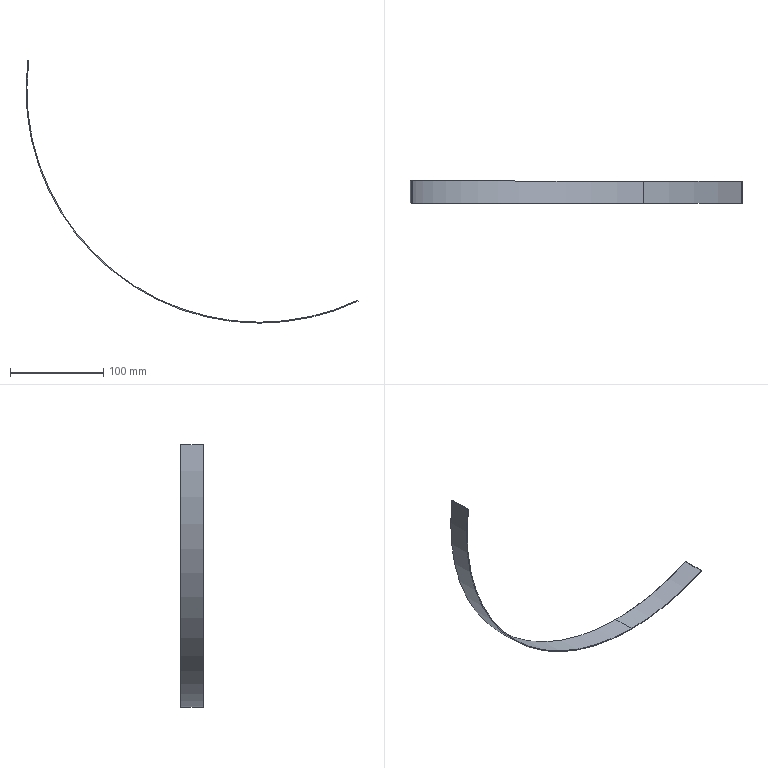Part | STEP file | 09-16 Track outer seal plate | 1 solid | 8 faces | box 357 x 24 x 282 mm | volume 12816 mm3 | cylinder 4 | plane 4 | commonest cylinder face diameters 500 x2 502 x2
STEP:
#1=CARTESIAN_POINT('',(0.,0.,0.));
#2=DIRECTION('',(0.,0.,1.));
#3=DIRECTION('',(1.,0.,0.));
#4=AXIS2_PLACEMENT_3D('',#1,#2,#3);
#5=CARTESIAN_POINT('',(106.,0.,-226.416));
#6=VERTEX_POINT('',#5);
#7=CARTESIAN_POINT('',(106.,24.,-226.416));
#8=VERTEX_POINT('',#7);
#9=CARTESIAN_POINT('',(106.,12.,-226.416));
#10=DIRECTION('',(0.,1.,0.));
#11=VECTOR('',#10,1.);
#12=LINE('',#9,#11);
#13=CARTESIAN_POINT('',(0.,24.,0.));
#14=DIRECTION('',(0.,-1.,0.));
#15=DIRECTION('',(0.,0.,-1.));
#16=AXIS2_PLACEMENT_3D('',#13,#14,#15);
#17=CYLINDRICAL_SURFACE('',#16,250.);
#18=CARTESIAN_POINT('',(0.4379,12.));
#19=DIRECTION('',(0.,-1.));
#20=VECTOR('',#19,1.);
#21=LINE('',#18,#20);
#22=(GEOMETRIC_REPRESENTATION_CONTEXT(2)PARAMETRIC_REPRESENTATION_CONTEXT()REPRESENTATION_CONTEXT('',''));
#23=DEFINITIONAL_REPRESENTATION('',(#21),#22);
#24=PCURVE('',#17,#23);
#25=CARTESIAN_POINT('',(106.,0.,-227.519));
#26=DIRECTION('',(-1.,0.,0.));
#27=DIRECTION('',(0.,0.,1.));
#28=AXIS2_PLACEMENT_3D('',#25,#26,#27);
#29=PLANE('',#28);
#30=CARTESIAN_POINT('',(1.104,12.));
#31=DIRECTION('',(0.,1.));
#32=VECTOR('',#31,1.);
#33=LINE('',#30,#32);
#34=(GEOMETRIC_REPRESENTATION_CONTEXT(2)PARAMETRIC_REPRESENTATION_CONTEXT()REPRESENTATION_CONTEXT('',''));
#35=DEFINITIONAL_REPRESENTATION('',(#33),#34);
#36=PCURVE('',#29,#35);
#37=SURFACE_CURVE('',#12,(#24,#36),.PCURVE_S1.);
#38=EDGE_CURVE('',#6,#8,#37,.T.);
#39=ORIENTED_EDGE('',*,*,#38,.F.);
#40=CARTESIAN_POINT('',(0.,0.,-250.));
#41=VERTEX_POINT('',#40);
#42=CARTESIAN_POINT('',(0.,0.,0.));
#43=DIRECTION('',(0.,-1.,0.));
#44=DIRECTION('',(0.,0.,-1.));
#45=AXIS2_PLACEMENT_3D('',#42,#43,#44);
#46=CIRCLE('',#45,250.);
#47=CARTESIAN_POINT('',(0.,24.));
#48=DIRECTION('',(1.,0.));
#49=VECTOR('',#48,1.);
#50=LINE('',#47,#49);
#51=(GEOMETRIC_REPRESENTATION_CONTEXT(2)PARAMETRIC_REPRESENTATION_CONTEXT()REPRESENTATION_CONTEXT('',''));
#52=DEFINITIONAL_REPRESENTATION('',(#50),#51);
#53=PCURVE('',#17,#52);
#54=CARTESIAN_POINT('',(-253.142,0.,-252.692));
#55=DIRECTION('',(0.,1.,0.));
#56=DIRECTION('',(0.,0.,1.));
#57=AXIS2_PLACEMENT_3D('',#54,#55,#56);
#58=PLANE('',#57);
#59=CARTESIAN_POINT('',(2.692,253.142));
#60=CARTESIAN_POINT('',(2.692,686.155));
#61=CARTESIAN_POINT('',(377.692,469.648));
#62=CARTESIAN_POINT('',(752.692,253.142));
#63=CARTESIAN_POINT('',(377.692,36.636));
#64=CARTESIAN_POINT('',(2.692,-179.871));
#65=CARTESIAN_POINT('',(2.692,253.142));
#66=(BOUNDED_CURVE()B_SPLINE_CURVE(2,(#59,#60,#61,#62,#63,#64,#65),.UNSPECIFIED.,.T.,.F.)B_SPLINE_CURVE_WITH_KNOTS((1,2,2,2,2,1),(-2.094,0.,2.094,4.189,6.283,8.378),.UNSPECIFIED.)CURVE()GEOMETRIC_REPRESENTATION_ITEM()RATIONAL_B_SPLINE_CURVE((1.,0.5,1.,0.5,1.,0.5,1.))REPRESENTATION_ITEM(''));
#67=(GEOMETRIC_REPRESENTATION_CONTEXT(2)PARAMETRIC_REPRESENTATION_CONTEXT()REPRESENTATION_CONTEXT('',''));
#68=DEFINITIONAL_REPRESENTATION('',(#66),#67);
#69=PCURVE('',#58,#68);
#70=SURFACE_CURVE('',#46,(#53,#69),.PCURVE_S1.);
#71=EDGE_CURVE('',#41,#6,#70,.T.);
#72=ORIENTED_EDGE('',*,*,#71,.F.);
#73=CARTESIAN_POINT('',(0.,24.,-250.));
#74=VERTEX_POINT('',#73);
#75=CARTESIAN_POINT('',(0.,24.,-250.));
#76=DIRECTION('',(0.,-1.,0.));
#77=VECTOR('',#76,1.);
#78=LINE('',#75,#77);
#79=CARTESIAN_POINT('',(0.,0.));
#80=DIRECTION('',(0.,1.));
#81=VECTOR('',#80,1.);
#82=LINE('',#79,#81);
#83=(GEOMETRIC_REPRESENTATION_CONTEXT(2)PARAMETRIC_REPRESENTATION_CONTEXT()REPRESENTATION_CONTEXT('',''));
#84=DEFINITIONAL_REPRESENTATION('',(#82),#83);
#85=PCURVE('',#17,#84);
#86=CARTESIAN_POINT('',(0.,24.,0.));
#87=DIRECTION('',(0.,-1.,0.));
#88=DIRECTION('',(0.,0.,-1.));
#89=AXIS2_PLACEMENT_3D('',#86,#87,#88);
#90=CYLINDRICAL_SURFACE('',#89,250.);
#91=CARTESIAN_POINT('',(6.283,0.));
#92=DIRECTION('',(0.,1.));
#93=VECTOR('',#92,1.);
#94=LINE('',#91,#93);
#95=(GEOMETRIC_REPRESENTATION_CONTEXT(2)PARAMETRIC_REPRESENTATION_CONTEXT()REPRESENTATION_CONTEXT('',''));
#96=DEFINITIONAL_REPRESENTATION('',(#94),#95);
#97=PCURVE('',#90,#96);
#98=SURFACE_CURVE('',#78,(#85,#97),.PCURVE_S1.);
#99=EDGE_CURVE('',#74,#41,#98,.T.);
#100=ORIENTED_EDGE('',*,*,#99,.F.);
#101=CARTESIAN_POINT('',(0.,24.,0.));
#102=DIRECTION('',(0.,1.,0.));
#103=DIRECTION('',(0.,0.,-1.));
#104=AXIS2_PLACEMENT_3D('',#101,#102,#103);
#105=CIRCLE('',#104,250.);
#106=CARTESIAN_POINT('',(6.283,0.));
#107=DIRECTION('',(-1.,0.));
#108=VECTOR('',#107,1.);
#109=LINE('',#106,#108);
#110=(GEOMETRIC_REPRESENTATION_CONTEXT(2)PARAMETRIC_REPRESENTATION_CONTEXT()REPRESENTATION_CONTEXT('',''));
#111=DEFINITIONAL_REPRESENTATION('',(#109),#110);
#112=PCURVE('',#17,#111);
#113=CARTESIAN_POINT('',(-253.142,24.,-252.692));
#114=DIRECTION('',(0.,1.,0.));
#115=DIRECTION('',(0.,0.,1.));
#116=AXIS2_PLACEMENT_3D('',#113,#114,#115);
#117=PLANE('',#116);
#118=CARTESIAN_POINT('',(252.692,253.142));
#119=DIRECTION('',(-1.,0.));
#120=AXIS2_PLACEMENT_2D('',#118,#119);
#121=CIRCLE('',#120,250.);
#122=(GEOMETRIC_REPRESENTATION_CONTEXT(2)PARAMETRIC_REPRESENTATION_CONTEXT()REPRESENTATION_CONTEXT('',''));
#123=DEFINITIONAL_REPRESENTATION('',(#121),#122);
#124=PCURVE('',#117,#123);
#125=SURFACE_CURVE('',#105,(#112,#124),.PCURVE_S1.);
#126=EDGE_CURVE('',#8,#74,#125,.T.);
#127=ORIENTED_EDGE('',*,*,#126,.F.);
#128=EDGE_LOOP('',(#39,#72,#100,#127));
#129=FACE_BOUND('',#128,.F.);
#130=ADVANCED_FACE('',(#129),#17,.F.);
#131=CARTESIAN_POINT('',(0.,24.,-251.));
#132=VERTEX_POINT('',#131);
#133=CARTESIAN_POINT('',(-249.078,24.,31.));
#134=VERTEX_POINT('',#133);
#135=CARTESIAN_POINT('',(0.,24.,0.));
#136=DIRECTION('',(0.,1.,0.));
#137=DIRECTION('',(0.,0.,-1.));
#138=AXIS2_PLACEMENT_3D('',#135,#136,#137);
#139=CIRCLE('',#138,251.);
#140=CARTESIAN_POINT('',(0.,24.,0.));
#141=DIRECTION('',(0.,-1.,0.));
#142=DIRECTION('',(0.,0.,-1.));
#143=AXIS2_PLACEMENT_3D('',#140,#141,#142);
#144=CYLINDRICAL_SURFACE('',#143,251.);
#145=CARTESIAN_POINT('',(6.283,0.));
#146=DIRECTION('',(-1.,0.));
#147=VECTOR('',#146,1.);
#148=LINE('',#145,#147);
#149=(GEOMETRIC_REPRESENTATION_CONTEXT(2)PARAMETRIC_REPRESENTATION_CONTEXT()REPRESENTATION_CONTEXT('',''));
#150=DEFINITIONAL_REPRESENTATION('',(#148),#149);
#151=PCURVE('',#144,#150);
#152=CARTESIAN_POINT('',(252.692,253.142));
#153=DIRECTION('',(-1.,0.));
#154=AXIS2_PLACEMENT_2D('',#152,#153);
#155=CIRCLE('',#154,251.);
#156=(GEOMETRIC_REPRESENTATION_CONTEXT(2)PARAMETRIC_REPRESENTATION_CONTEXT()REPRESENTATION_CONTEXT('',''));
#157=DEFINITIONAL_REPRESENTATION('',(#155),#156);
#158=PCURVE('',#117,#157);
#159=SURFACE_CURVE('',#139,(#151,#158),.PCURVE_S1.);
#160=EDGE_CURVE('',#132,#134,#159,.T.);
#161=ORIENTED_EDGE('',*,*,#160,.F.);
#162=CARTESIAN_POINT('',(0.,0.,-251.));
#163=VERTEX_POINT('',#162);
#164=CARTESIAN_POINT('',(0.,24.,-251.));
#165=DIRECTION('',(0.,-1.,0.));
#166=VECTOR('',#165,1.);
#167=LINE('',#164,#166);
#168=CARTESIAN_POINT('',(6.283,0.));
#169=DIRECTION('',(0.,1.));
#170=VECTOR('',#169,1.);
#171=LINE('',#168,#170);
#172=(GEOMETRIC_REPRESENTATION_CONTEXT(2)PARAMETRIC_REPRESENTATION_CONTEXT()REPRESENTATION_CONTEXT('',''));
#173=DEFINITIONAL_REPRESENTATION('',(#171),#172);
#174=PCURVE('',#144,#173);
#175=CARTESIAN_POINT('',(0.,24.,0.));
#176=DIRECTION('',(0.,-1.,0.));
#177=DIRECTION('',(0.,0.,-1.));
#178=AXIS2_PLACEMENT_3D('',#175,#176,#177);
#179=CYLINDRICAL_SURFACE('',#178,251.);
#180=CARTESIAN_POINT('',(0.,0.));
#181=DIRECTION('',(0.,1.));
#182=VECTOR('',#181,1.);
#183=LINE('',#180,#182);
#184=(GEOMETRIC_REPRESENTATION_CONTEXT(2)PARAMETRIC_REPRESENTATION_CONTEXT()REPRESENTATION_CONTEXT('',''));
#185=DEFINITIONAL_REPRESENTATION('',(#183),#184);
#186=PCURVE('',#179,#185);
#187=SURFACE_CURVE('',#167,(#174,#186),.PCURVE_S1.);
#188=EDGE_CURVE('',#132,#163,#187,.T.);
#189=ORIENTED_EDGE('',*,*,#188,.T.);
#190=CARTESIAN_POINT('',(-249.078,0.,31.));
#191=VERTEX_POINT('',#190);
#192=CARTESIAN_POINT('',(0.,0.,0.));
#193=DIRECTION('',(0.,1.,0.));
#194=DIRECTION('',(0.,0.,-1.));
#195=AXIS2_PLACEMENT_3D('',#192,#193,#194);
#196=CIRCLE('',#195,251.);
#197=CARTESIAN_POINT('',(6.283,24.));
#198=DIRECTION('',(-1.,0.));
#199=VECTOR('',#198,1.);
#200=LINE('',#197,#199);
#201=(GEOMETRIC_REPRESENTATION_CONTEXT(2)PARAMETRIC_REPRESENTATION_CONTEXT()REPRESENTATION_CONTEXT('',''));
#202=DEFINITIONAL_REPRESENTATION('',(#200),#201);
#203=PCURVE('',#144,#202);
#204=CARTESIAN_POINT('',(252.692,253.142));
#205=DIRECTION('',(-1.,0.));
#206=AXIS2_PLACEMENT_2D('',#204,#205);
#207=CIRCLE('',#206,251.);
#208=(GEOMETRIC_REPRESENTATION_CONTEXT(2)PARAMETRIC_REPRESENTATION_CONTEXT()REPRESENTATION_CONTEXT('',''));
#209=DEFINITIONAL_REPRESENTATION('',(#207),#208);
#210=PCURVE('',#58,#209);
#211=SURFACE_CURVE('',#196,(#203,#210),.PCURVE_S1.);
#212=EDGE_CURVE('',#163,#191,#211,.T.);
#213=ORIENTED_EDGE('',*,*,#212,.T.);
#214=CARTESIAN_POINT('',(-249.078,12.,31.));
#215=DIRECTION('',(0.,-1.,0.));
#216=VECTOR('',#215,1.);
#217=LINE('',#214,#216);
#218=CARTESIAN_POINT('',(4.589,12.));
#219=DIRECTION('',(0.,1.));
#220=VECTOR('',#219,1.);
#221=LINE('',#218,#220);
#222=(GEOMETRIC_REPRESENTATION_CONTEXT(2)PARAMETRIC_REPRESENTATION_CONTEXT()REPRESENTATION_CONTEXT('',''));
#223=DEFINITIONAL_REPRESENTATION('',(#221),#222);
#224=PCURVE('',#144,#223);
#225=CARTESIAN_POINT('',(-248.071,0.,31.));
#226=DIRECTION('',(0.,0.,-1.));
#227=DIRECTION('',(-1.,0.,0.));
#228=AXIS2_PLACEMENT_3D('',#225,#226,#227);
#229=PLANE('',#228);
#230=CARTESIAN_POINT('',(1.008,12.));
#231=DIRECTION('',(0.,-1.));
#232=VECTOR('',#231,1.);
#233=LINE('',#230,#232);
#234=(GEOMETRIC_REPRESENTATION_CONTEXT(2)PARAMETRIC_REPRESENTATION_CONTEXT()REPRESENTATION_CONTEXT('',''));
#235=DEFINITIONAL_REPRESENTATION('',(#233),#234);
#236=PCURVE('',#229,#235);
#237=SURFACE_CURVE('',#217,(#224,#236),.PCURVE_S1.);
#238=EDGE_CURVE('',#134,#191,#237,.T.);
#239=ORIENTED_EDGE('',*,*,#238,.F.);
#240=EDGE_LOOP('',(#161,#189,#213,#239));
#241=FACE_BOUND('',#240,.T.);
#242=ADVANCED_FACE('',(#241),#144,.T.);
#243=CARTESIAN_POINT('',(-248.071,0.,31.));
#244=VERTEX_POINT('',#243);
#245=CARTESIAN_POINT('',(0.,0.,0.));
#246=DIRECTION('',(0.,-1.,0.));
#247=DIRECTION('',(0.,0.,-1.));
#248=AXIS2_PLACEMENT_3D('',#245,#246,#247);
#249=CIRCLE('',#248,250.);
#250=CARTESIAN_POINT('',(0.,24.));
#251=DIRECTION('',(1.,0.));
#252=VECTOR('',#251,1.);
#253=LINE('',#250,#252);
#254=(GEOMETRIC_REPRESENTATION_CONTEXT(2)PARAMETRIC_REPRESENTATION_CONTEXT()REPRESENTATION_CONTEXT('',''));
#255=DEFINITIONAL_REPRESENTATION('',(#253),#254);
#256=PCURVE('',#90,#255);
#257=CARTESIAN_POINT('',(2.692,253.142));
#258=CARTESIAN_POINT('',(2.692,686.155));
#259=CARTESIAN_POINT('',(377.692,469.648));
#260=CARTESIAN_POINT('',(752.692,253.142));
#261=CARTESIAN_POINT('',(377.692,36.636));
#262=CARTESIAN_POINT('',(2.692,-179.871));
#263=CARTESIAN_POINT('',(2.692,253.142));
#264=(BOUNDED_CURVE()B_SPLINE_CURVE(2,(#257,#258,#259,#260,#261,#262,#263),.UNSPECIFIED.,.T.,.F.)B_SPLINE_CURVE_WITH_KNOTS((1,2,2,2,2,1),(-2.094,0.,2.094,4.189,6.283,8.378),.UNSPECIFIED.)CURVE()GEOMETRIC_REPRESENTATION_ITEM()RATIONAL_B_SPLINE_CURVE((1.,0.5,1.,0.5,1.,0.5,1.))REPRESENTATION_ITEM(''));
#265=(GEOMETRIC_REPRESENTATION_CONTEXT(2)PARAMETRIC_REPRESENTATION_CONTEXT()REPRESENTATION_CONTEXT('',''));
#266=DEFINITIONAL_REPRESENTATION('',(#264),#265);
#267=PCURVE('',#58,#266);
#268=SURFACE_CURVE('',#249,(#256,#267),.PCURVE_S1.);
#269=EDGE_CURVE('',#244,#41,#268,.T.);
#270=ORIENTED_EDGE('',*,*,#269,.F.);
#271=CARTESIAN_POINT('',(-248.071,24.,31.));
#272=VERTEX_POINT('',#271);
#273=CARTESIAN_POINT('',(-248.071,12.,31.));
#274=DIRECTION('',(0.,-1.,0.));
#275=VECTOR('',#274,1.);
#276=LINE('',#273,#275);
#277=CARTESIAN_POINT('',(4.588,12.));
#278=DIRECTION('',(0.,1.));
#279=VECTOR('',#278,1.);
#280=LINE('',#277,#279);
#281=(GEOMETRIC_REPRESENTATION_CONTEXT(2)PARAMETRIC_REPRESENTATION_CONTEXT()REPRESENTATION_CONTEXT('',''));
#282=DEFINITIONAL_REPRESENTATION('',(#280),#281);
#283=PCURVE('',#90,#282);
#284=CARTESIAN_POINT('',(0.00000001,12.));
#285=DIRECTION('',(0.,-1.));
#286=VECTOR('',#285,1.);
#287=LINE('',#284,#286);
#288=(GEOMETRIC_REPRESENTATION_CONTEXT(2)PARAMETRIC_REPRESENTATION_CONTEXT()REPRESENTATION_CONTEXT('',''));
#289=DEFINITIONAL_REPRESENTATION('',(#287),#288);
#290=PCURVE('',#229,#289);
#291=SURFACE_CURVE('',#276,(#283,#290),.PCURVE_S1.);
#292=EDGE_CURVE('',#272,#244,#291,.T.);
#293=ORIENTED_EDGE('',*,*,#292,.F.);
#294=CARTESIAN_POINT('',(0.,24.,0.));
#295=DIRECTION('',(0.,1.,0.));
#296=DIRECTION('',(0.,0.,-1.));
#297=AXIS2_PLACEMENT_3D('',#294,#295,#296);
#298=CIRCLE('',#297,250.);
#299=CARTESIAN_POINT('',(6.283,0.));
#300=DIRECTION('',(-1.,0.));
#301=VECTOR('',#300,1.);
#302=LINE('',#299,#301);
#303=(GEOMETRIC_REPRESENTATION_CONTEXT(2)PARAMETRIC_REPRESENTATION_CONTEXT()REPRESENTATION_CONTEXT('',''));
#304=DEFINITIONAL_REPRESENTATION('',(#302),#303);
#305=PCURVE('',#90,#304);
#306=CARTESIAN_POINT('',(252.692,253.142));
#307=DIRECTION('',(-1.,0.));
#308=AXIS2_PLACEMENT_2D('',#306,#307);
#309=CIRCLE('',#308,250.);
#310=(GEOMETRIC_REPRESENTATION_CONTEXT(2)PARAMETRIC_REPRESENTATION_CONTEXT()REPRESENTATION_CONTEXT('',''));
#311=DEFINITIONAL_REPRESENTATION('',(#309),#310);
#312=PCURVE('',#117,#311);
#313=SURFACE_CURVE('',#298,(#305,#312),.PCURVE_S1.);
#314=EDGE_CURVE('',#74,#272,#313,.T.);
#315=ORIENTED_EDGE('',*,*,#314,.F.);
#316=ORIENTED_EDGE('',*,*,#99,.T.);
#317=EDGE_LOOP('',(#270,#293,#315,#316));
#318=FACE_BOUND('',#317,.F.);
#319=ADVANCED_FACE('',(#318),#90,.F.);
#320=CARTESIAN_POINT('',(106.,24.,-227.519));
#321=VERTEX_POINT('',#320);
#322=CARTESIAN_POINT('',(106.,0.,-227.519));
#323=VERTEX_POINT('',#322);
#324=CARTESIAN_POINT('',(106.,12.,-227.519));
#325=DIRECTION('',(0.,-1.,0.));
#326=VECTOR('',#325,1.);
#327=LINE('',#324,#326);
#328=CARTESIAN_POINT('',(0.,12.));
#329=DIRECTION('',(0.,-1.));
#330=VECTOR('',#329,1.);
#331=LINE('',#328,#330);
#332=(GEOMETRIC_REPRESENTATION_CONTEXT(2)PARAMETRIC_REPRESENTATION_CONTEXT()REPRESENTATION_CONTEXT('',''));
#333=DEFINITIONAL_REPRESENTATION('',(#331),#332);
#334=PCURVE('',#29,#333);
#335=CARTESIAN_POINT('',(0.436,12.));
#336=DIRECTION('',(0.,1.));
#337=VECTOR('',#336,1.);
#338=LINE('',#335,#337);
#339=(GEOMETRIC_REPRESENTATION_CONTEXT(2)PARAMETRIC_REPRESENTATION_CONTEXT()REPRESENTATION_CONTEXT('',''));
#340=DEFINITIONAL_REPRESENTATION('',(#338),#339);
#341=PCURVE('',#179,#340);
#342=SURFACE_CURVE('',#327,(#334,#341),.PCURVE_S1.);
#343=EDGE_CURVE('',#321,#323,#342,.T.);
#344=ORIENTED_EDGE('',*,*,#343,.F.);
#345=CARTESIAN_POINT('',(106.,24.,-226.967));
#346=DIRECTION('',(0.,0.,-1.));
#347=VECTOR('',#346,1.);
#348=LINE('',#345,#347);
#349=CARTESIAN_POINT('',(0.5518,24.));
#350=DIRECTION('',(-1.,0.));
#351=VECTOR('',#350,1.);
#352=LINE('',#349,#351);
#353=(GEOMETRIC_REPRESENTATION_CONTEXT(2)PARAMETRIC_REPRESENTATION_CONTEXT()REPRESENTATION_CONTEXT('',''));
#354=DEFINITIONAL_REPRESENTATION('',(#352),#353);
#355=PCURVE('',#29,#354);
#356=CARTESIAN_POINT('',(25.725,359.142));
#357=DIRECTION('',(-1.,0.));
#358=VECTOR('',#357,1.);
#359=LINE('',#356,#358);
#360=(GEOMETRIC_REPRESENTATION_CONTEXT(2)PARAMETRIC_REPRESENTATION_CONTEXT()REPRESENTATION_CONTEXT('',''));
#361=DEFINITIONAL_REPRESENTATION('',(#359),#360);
#362=PCURVE('',#117,#361);
#363=SURFACE_CURVE('',#348,(#355,#362),.PCURVE_S1.);
#364=EDGE_CURVE('',#8,#321,#363,.T.);
#365=ORIENTED_EDGE('',*,*,#364,.F.);
#366=ORIENTED_EDGE('',*,*,#38,.F.);
#367=CARTESIAN_POINT('',(106.,0.,-226.967));
#368=DIRECTION('',(0.,0.,1.));
#369=VECTOR('',#368,1.);
#370=LINE('',#367,#369);
#371=CARTESIAN_POINT('',(0.5518,0.));
#372=DIRECTION('',(1.,0.));
#373=VECTOR('',#372,1.);
#374=LINE('',#371,#373);
#375=(GEOMETRIC_REPRESENTATION_CONTEXT(2)PARAMETRIC_REPRESENTATION_CONTEXT()REPRESENTATION_CONTEXT('',''));
#376=DEFINITIONAL_REPRESENTATION('',(#374),#375);
#377=PCURVE('',#29,#376);
#378=CARTESIAN_POINT('',(25.725,359.142));
#379=DIRECTION('',(1.,0.));
#380=VECTOR('',#379,1.);
#381=LINE('',#378,#380);
#382=(GEOMETRIC_REPRESENTATION_CONTEXT(2)PARAMETRIC_REPRESENTATION_CONTEXT()REPRESENTATION_CONTEXT('',''));
#383=DEFINITIONAL_REPRESENTATION('',(#381),#382);
#384=PCURVE('',#58,#383);
#385=SURFACE_CURVE('',#370,(#377,#384),.PCURVE_S1.);
#386=EDGE_CURVE('',#323,#6,#385,.T.);
#387=ORIENTED_EDGE('',*,*,#386,.F.);
#388=EDGE_LOOP('',(#344,#365,#366,#387));
#389=FACE_BOUND('',#388,.T.);
#390=ADVANCED_FACE('',(#389),#29,.F.);
#391=ORIENTED_EDGE('',*,*,#386,.T.);
#392=ORIENTED_EDGE('',*,*,#71,.F.);
#393=ORIENTED_EDGE('',*,*,#269,.F.);
#394=CARTESIAN_POINT('',(-248.574,0.,31.));
#395=DIRECTION('',(-1.,0.,0.));
#396=VECTOR('',#395,1.);
#397=LINE('',#394,#396);
#398=CARTESIAN_POINT('',(283.692,4.568));
#399=DIRECTION('',(0.,-1.));
#400=VECTOR('',#399,1.);
#401=LINE('',#398,#400);
#402=(GEOMETRIC_REPRESENTATION_CONTEXT(2)PARAMETRIC_REPRESENTATION_CONTEXT()REPRESENTATION_CONTEXT('',''));
#403=DEFINITIONAL_REPRESENTATION('',(#401),#402);
#404=PCURVE('',#58,#403);
#405=CARTESIAN_POINT('',(0.5039,0.));
#406=DIRECTION('',(1.,0.));
#407=VECTOR('',#406,1.);
#408=LINE('',#405,#407);
#409=(GEOMETRIC_REPRESENTATION_CONTEXT(2)PARAMETRIC_REPRESENTATION_CONTEXT()REPRESENTATION_CONTEXT('',''));
#410=DEFINITIONAL_REPRESENTATION('',(#408),#409);
#411=PCURVE('',#229,#410);
#412=SURFACE_CURVE('',#397,(#404,#411),.PCURVE_S1.);
#413=EDGE_CURVE('',#244,#191,#412,.T.);
#414=ORIENTED_EDGE('',*,*,#413,.T.);
#415=ORIENTED_EDGE('',*,*,#212,.F.);
#416=CARTESIAN_POINT('',(0.,0.,0.));
#417=DIRECTION('',(0.,1.,0.));
#418=DIRECTION('',(0.,0.,-1.));
#419=AXIS2_PLACEMENT_3D('',#416,#417,#418);
#420=CIRCLE('',#419,251.);
#421=CARTESIAN_POINT('',(252.692,253.142));
#422=DIRECTION('',(-1.,0.));
#423=AXIS2_PLACEMENT_2D('',#421,#422);
#424=CIRCLE('',#423,251.);
#425=(GEOMETRIC_REPRESENTATION_CONTEXT(2)PARAMETRIC_REPRESENTATION_CONTEXT()REPRESENTATION_CONTEXT('',''));
#426=DEFINITIONAL_REPRESENTATION('',(#424),#425);
#427=PCURVE('',#58,#426);
#428=CARTESIAN_POINT('',(6.283,24.));
#429=DIRECTION('',(-1.,0.));
#430=VECTOR('',#429,1.);
#431=LINE('',#428,#430);
#432=(GEOMETRIC_REPRESENTATION_CONTEXT(2)PARAMETRIC_REPRESENTATION_CONTEXT()REPRESENTATION_CONTEXT('',''));
#433=DEFINITIONAL_REPRESENTATION('',(#431),#432);
#434=PCURVE('',#179,#433);
#435=SURFACE_CURVE('',#420,(#427,#434),.PCURVE_S1.);
#436=EDGE_CURVE('',#323,#163,#435,.T.);
#437=ORIENTED_EDGE('',*,*,#436,.F.);
#438=EDGE_LOOP('',(#391,#392,#393,#414,#415,#437));
#439=FACE_BOUND('',#438,.T.);
#440=ADVANCED_FACE('',(#439),#58,.F.);
#441=ORIENTED_EDGE('',*,*,#126,.F.);
#442=ORIENTED_EDGE('',*,*,#364,.T.);
#443=CARTESIAN_POINT('',(0.,24.,0.));
#444=DIRECTION('',(0.,1.,0.));
#445=DIRECTION('',(0.,0.,-1.));
#446=AXIS2_PLACEMENT_3D('',#443,#444,#445);
#447=CIRCLE('',#446,251.);
#448=CARTESIAN_POINT('',(252.692,253.142));
#449=DIRECTION('',(-1.,0.));
#450=AXIS2_PLACEMENT_2D('',#448,#449);
#451=CIRCLE('',#450,251.);
#452=(GEOMETRIC_REPRESENTATION_CONTEXT(2)PARAMETRIC_REPRESENTATION_CONTEXT()REPRESENTATION_CONTEXT('',''));
#453=DEFINITIONAL_REPRESENTATION('',(#451),#452);
#454=PCURVE('',#117,#453);
#455=CARTESIAN_POINT('',(6.283,0.));
#456=DIRECTION('',(-1.,0.));
#457=VECTOR('',#456,1.);
#458=LINE('',#455,#457);
#459=(GEOMETRIC_REPRESENTATION_CONTEXT(2)PARAMETRIC_REPRESENTATION_CONTEXT()REPRESENTATION_CONTEXT('',''));
#460=DEFINITIONAL_REPRESENTATION('',(#458),#459);
#461=PCURVE('',#179,#460);
#462=SURFACE_CURVE('',#447,(#454,#461),.PCURVE_S1.);
#463=EDGE_CURVE('',#321,#132,#462,.T.);
#464=ORIENTED_EDGE('',*,*,#463,.T.);
#465=ORIENTED_EDGE('',*,*,#160,.T.);
#466=CARTESIAN_POINT('',(-73.571,24.,31.));
#467=DIRECTION('',(1.,0.,0.));
#468=VECTOR('',#467,1.);
#469=LINE('',#466,#468);
#470=CARTESIAN_POINT('',(283.692,179.571));
#471=DIRECTION('',(0.,1.));
#472=VECTOR('',#471,1.);
#473=LINE('',#470,#472);
#474=(GEOMETRIC_REPRESENTATION_CONTEXT(2)PARAMETRIC_REPRESENTATION_CONTEXT()REPRESENTATION_CONTEXT('',''));
#475=DEFINITIONAL_REPRESENTATION('',(#473),#474);
#476=PCURVE('',#117,#475);
#477=CARTESIAN_POINT('',(-174.5,24.));
#478=DIRECTION('',(-1.,0.));
#479=VECTOR('',#478,1.);
#480=LINE('',#477,#479);
#481=(GEOMETRIC_REPRESENTATION_CONTEXT(2)PARAMETRIC_REPRESENTATION_CONTEXT()REPRESENTATION_CONTEXT('',''));
#482=DEFINITIONAL_REPRESENTATION('',(#480),#481);
#483=PCURVE('',#229,#482);
#484=SURFACE_CURVE('',#469,(#476,#483),.PCURVE_S1.);
#485=EDGE_CURVE('',#134,#272,#484,.T.);
#486=ORIENTED_EDGE('',*,*,#485,.T.);
#487=ORIENTED_EDGE('',*,*,#314,.F.);
#488=EDGE_LOOP('',(#441,#442,#464,#465,#486,#487));
#489=FACE_BOUND('',#488,.T.);
#490=ADVANCED_FACE('',(#489),#117,.T.);
#491=ORIENTED_EDGE('',*,*,#188,.F.);
#492=ORIENTED_EDGE('',*,*,#463,.F.);
#493=ORIENTED_EDGE('',*,*,#343,.T.);
#494=ORIENTED_EDGE('',*,*,#436,.T.);
#495=EDGE_LOOP('',(#491,#492,#493,#494));
#496=FACE_BOUND('',#495,.T.);
#497=ADVANCED_FACE('',(#496),#179,.T.);
#498=ORIENTED_EDGE('',*,*,#292,.F.);
#499=ORIENTED_EDGE('',*,*,#485,.F.);
#500=ORIENTED_EDGE('',*,*,#238,.T.);
#501=ORIENTED_EDGE('',*,*,#413,.F.);
#502=EDGE_LOOP('',(#498,#499,#500,#501));
#503=FACE_BOUND('',#502,.T.);
#504=ADVANCED_FACE('',(#503),#229,.F.);
#505=CLOSED_SHELL('',(#130,#242,#319,#390,#440,#490,#497,#504));
#506=MANIFOLD_SOLID_BREP('',#505);
#507=(LENGTH_UNIT()NAMED_UNIT(*)SI_UNIT(.MILLI.,.METRE.));
#508=UNCERTAINTY_MEASURE_WITH_UNIT(LENGTH_MEASURE(0.0000001),#507,'','');
#509=(NAMED_UNIT(*)PLANE_ANGLE_UNIT()SI_UNIT($,.RADIAN.));
#510=(NAMED_UNIT(*)SI_UNIT($,.STERADIAN.)SOLID_ANGLE_UNIT());
#511=(GEOMETRIC_REPRESENTATION_CONTEXT(3)GLOBAL_UNCERTAINTY_ASSIGNED_CONTEXT((#508))GLOBAL_UNIT_ASSIGNED_CONTEXT((#507,#509,#510))REPRESENTATION_CONTEXT('',''));
#512=ADVANCED_BREP_SHAPE_REPRESENTATION('',(#4,#506),#511);